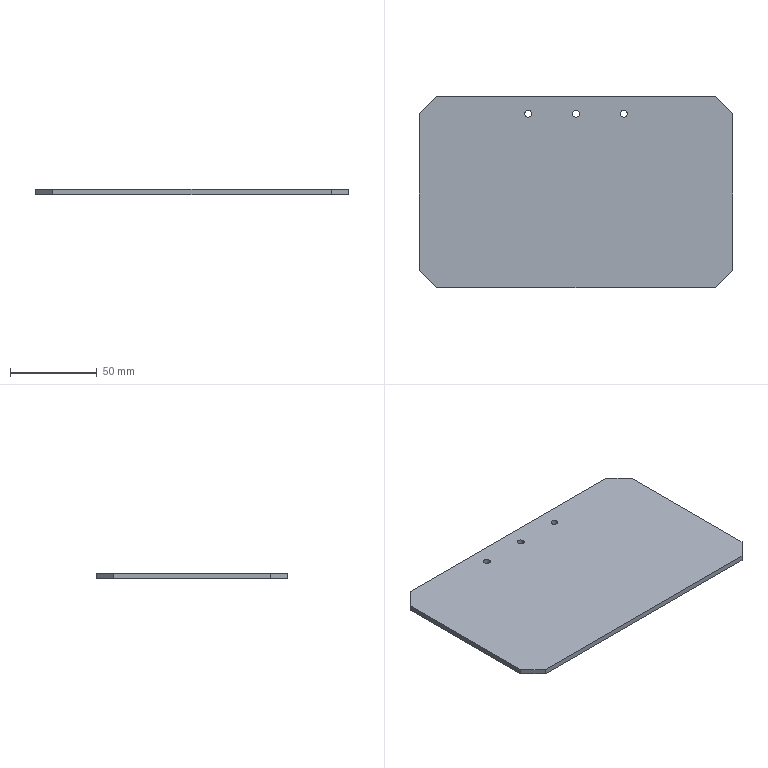Part | SolidWorks | features Extrusion 1 | 1 solid | 16 faces | box 180 x 110 x 3 mm | volume 58687 mm3 | plane 10 | cylinder 6 | commonest cylinder face diameters 4 x6
STEP:
#1=CARTESIAN_POINT('',(60.5,-10.,3.));
#2=VERTEX_POINT('',#1);
#3=CARTESIAN_POINT('',(64.5,-10.,3.));
#4=VERTEX_POINT('',#3);
#5=CARTESIAN_POINT('',(62.5,-10.,3.));
#6=DIRECTION('',(0.,0.,1.));
#7=DIRECTION('',(1.,0.,0.));
#8=AXIS2_PLACEMENT_3D('',#5,#6,#7);
#9=CIRCLE('',#8,2.);
#10=EDGE_CURVE('',#2,#4,#9,.T.);
#11=ORIENTED_EDGE('',*,*,#10,.T.);
#12=CARTESIAN_POINT('',(64.5,-10.,0.));
#13=VERTEX_POINT('',#12);
#14=CARTESIAN_POINT('',(64.5,-10.,3.));
#15=DIRECTION('',(0.,0.,-1.));
#16=VECTOR('',#15,1000.);
#17=LINE('',#14,#16);
#18=EDGE_CURVE('',#4,#13,#17,.T.);
#19=ORIENTED_EDGE('',*,*,#18,.T.);
#20=CARTESIAN_POINT('',(60.5,-10.,0.));
#21=VERTEX_POINT('',#20);
#22=CARTESIAN_POINT('',(62.5,-10.,0.));
#23=DIRECTION('',(0.,0.,1.));
#24=DIRECTION('',(1.,0.,0.));
#25=AXIS2_PLACEMENT_3D('',#22,#23,#24);
#26=CIRCLE('',#25,2.);
#27=EDGE_CURVE('',#21,#13,#26,.T.);
#28=ORIENTED_EDGE('',*,*,#27,.F.);
#29=CARTESIAN_POINT('',(60.5,-10.,3.));
#30=DIRECTION('',(0.,0.,-1.));
#31=VECTOR('',#30,1000.);
#32=LINE('',#29,#31);
#33=EDGE_CURVE('',#2,#21,#32,.T.);
#34=ORIENTED_EDGE('',*,*,#33,.F.);
#35=EDGE_LOOP('',(#11,#19,#28,#34));
#36=FACE_OUTER_BOUND('',#35,.T.);
#37=CARTESIAN_POINT('',(62.5,-10.,3.));
#38=DIRECTION('',(0.,0.,-1.));
#39=DIRECTION('',(-1.,0.,0.));
#40=AXIS2_PLACEMENT_3D('',#37,#38,#39);
#41=CYLINDRICAL_SURFACE('',#40,2.);
#42=ADVANCED_FACE('',(#36),#41,.F.);
#43=CARTESIAN_POINT('',(115.5,-10.,3.));
#44=VERTEX_POINT('',#43);
#45=CARTESIAN_POINT('',(119.5,-10.,3.));
#46=VERTEX_POINT('',#45);
#47=CARTESIAN_POINT('',(117.5,-10.,3.));
#48=DIRECTION('',(0.,0.,1.));
#49=DIRECTION('',(1.,0.,0.));
#50=AXIS2_PLACEMENT_3D('',#47,#48,#49);
#51=CIRCLE('',#50,2.);
#52=EDGE_CURVE('',#44,#46,#51,.T.);
#53=ORIENTED_EDGE('',*,*,#52,.T.);
#54=CARTESIAN_POINT('',(119.5,-10.,0.));
#55=VERTEX_POINT('',#54);
#56=CARTESIAN_POINT('',(119.5,-10.,3.));
#57=DIRECTION('',(0.,0.,-1.));
#58=VECTOR('',#57,1000.);
#59=LINE('',#56,#58);
#60=EDGE_CURVE('',#46,#55,#59,.T.);
#61=ORIENTED_EDGE('',*,*,#60,.T.);
#62=CARTESIAN_POINT('',(115.5,-10.,0.));
#63=VERTEX_POINT('',#62);
#64=CARTESIAN_POINT('',(117.5,-10.,0.));
#65=DIRECTION('',(0.,0.,1.));
#66=DIRECTION('',(1.,0.,0.));
#67=AXIS2_PLACEMENT_3D('',#64,#65,#66);
#68=CIRCLE('',#67,2.);
#69=EDGE_CURVE('',#63,#55,#68,.T.);
#70=ORIENTED_EDGE('',*,*,#69,.F.);
#71=CARTESIAN_POINT('',(115.5,-10.,3.));
#72=DIRECTION('',(0.,0.,-1.));
#73=VECTOR('',#72,1000.);
#74=LINE('',#71,#73);
#75=EDGE_CURVE('',#44,#63,#74,.T.);
#76=ORIENTED_EDGE('',*,*,#75,.F.);
#77=EDGE_LOOP('',(#53,#61,#70,#76));
#78=FACE_OUTER_BOUND('',#77,.T.);
#79=CARTESIAN_POINT('',(117.5,-10.,3.));
#80=DIRECTION('',(0.,0.,-1.));
#81=DIRECTION('',(-1.,0.,0.));
#82=AXIS2_PLACEMENT_3D('',#79,#80,#81);
#83=CYLINDRICAL_SURFACE('',#82,2.);
#84=ADVANCED_FACE('',(#78),#83,.F.);
#85=CARTESIAN_POINT('',(88.,-10.,3.));
#86=VERTEX_POINT('',#85);
#87=CARTESIAN_POINT('',(92.,-10.,3.));
#88=VERTEX_POINT('',#87);
#89=CARTESIAN_POINT('',(90.,-10.,3.));
#90=DIRECTION('',(0.,0.,1.));
#91=DIRECTION('',(1.,0.,0.));
#92=AXIS2_PLACEMENT_3D('',#89,#90,#91);
#93=CIRCLE('',#92,2.);
#94=EDGE_CURVE('',#86,#88,#93,.T.);
#95=ORIENTED_EDGE('',*,*,#94,.T.);
#96=CARTESIAN_POINT('',(92.,-10.,0.));
#97=VERTEX_POINT('',#96);
#98=CARTESIAN_POINT('',(92.,-10.,3.));
#99=DIRECTION('',(0.,0.,-1.));
#100=VECTOR('',#99,1000.);
#101=LINE('',#98,#100);
#102=EDGE_CURVE('',#88,#97,#101,.T.);
#103=ORIENTED_EDGE('',*,*,#102,.T.);
#104=CARTESIAN_POINT('',(88.,-10.,0.));
#105=VERTEX_POINT('',#104);
#106=CARTESIAN_POINT('',(90.,-10.,0.));
#107=DIRECTION('',(0.,0.,1.));
#108=DIRECTION('',(1.,0.,0.));
#109=AXIS2_PLACEMENT_3D('',#106,#107,#108);
#110=CIRCLE('',#109,2.);
#111=EDGE_CURVE('',#105,#97,#110,.T.);
#112=ORIENTED_EDGE('',*,*,#111,.F.);
#113=CARTESIAN_POINT('',(88.,-10.,3.));
#114=DIRECTION('',(0.,0.,-1.));
#115=VECTOR('',#114,1000.);
#116=LINE('',#113,#115);
#117=EDGE_CURVE('',#86,#105,#116,.T.);
#118=ORIENTED_EDGE('',*,*,#117,.F.);
#119=EDGE_LOOP('',(#95,#103,#112,#118));
#120=FACE_OUTER_BOUND('',#119,.T.);
#121=CARTESIAN_POINT('',(90.,-10.,3.));
#122=DIRECTION('',(0.,0.,-1.));
#123=DIRECTION('',(-1.,0.,0.));
#124=AXIS2_PLACEMENT_3D('',#121,#122,#123);
#125=CYLINDRICAL_SURFACE('',#124,2.);
#126=ADVANCED_FACE('',(#120),#125,.F.);
#127=ORIENTED_EDGE('',*,*,#52,.F.);
#128=CARTESIAN_POINT('',(117.5,-10.,3.));
#129=DIRECTION('',(0.,0.,1.));
#130=DIRECTION('',(1.,0.,0.));
#131=AXIS2_PLACEMENT_3D('',#128,#129,#130);
#132=CIRCLE('',#131,2.);
#133=EDGE_CURVE('',#46,#44,#132,.T.);
#134=ORIENTED_EDGE('',*,*,#133,.F.);
#135=EDGE_LOOP('',(#127,#134));
#136=FACE_BOUND('',#135,.T.);
#137=CARTESIAN_POINT('',(10.,0.,3.));
#138=VERTEX_POINT('',#137);
#139=CARTESIAN_POINT('',(0.,-10.,3.));
#140=VERTEX_POINT('',#139);
#141=CARTESIAN_POINT('',(10.,0.,3.));
#142=DIRECTION('',(-0.7071,-0.7071,0.));
#143=VECTOR('',#142,1000.);
#144=LINE('',#141,#143);
#145=EDGE_CURVE('',#138,#140,#144,.T.);
#146=ORIENTED_EDGE('',*,*,#145,.T.);
#147=CARTESIAN_POINT('',(0.,-100.,3.));
#148=VERTEX_POINT('',#147);
#149=CARTESIAN_POINT('',(0.,-10.,3.));
#150=DIRECTION('',(0.,-1.,0.));
#151=VECTOR('',#150,1000.);
#152=LINE('',#149,#151);
#153=EDGE_CURVE('',#140,#148,#152,.T.);
#154=ORIENTED_EDGE('',*,*,#153,.T.);
#155=CARTESIAN_POINT('',(10.,-110.,3.));
#156=VERTEX_POINT('',#155);
#157=CARTESIAN_POINT('',(0.,-100.,3.));
#158=DIRECTION('',(0.7071,-0.7071,0.));
#159=VECTOR('',#158,1000.);
#160=LINE('',#157,#159);
#161=EDGE_CURVE('',#148,#156,#160,.T.);
#162=ORIENTED_EDGE('',*,*,#161,.T.);
#163=CARTESIAN_POINT('',(170.,-110.,3.));
#164=VERTEX_POINT('',#163);
#165=CARTESIAN_POINT('',(10.,-110.,3.));
#166=DIRECTION('',(1.,0.,0.));
#167=VECTOR('',#166,1000.);
#168=LINE('',#165,#167);
#169=EDGE_CURVE('',#156,#164,#168,.T.);
#170=ORIENTED_EDGE('',*,*,#169,.T.);
#171=CARTESIAN_POINT('',(180.,-100.,3.));
#172=VERTEX_POINT('',#171);
#173=CARTESIAN_POINT('',(180.,-100.,3.));
#174=DIRECTION('',(0.7071,0.7071,0.));
#175=VECTOR('',#174,1000.);
#176=LINE('',#173,#175);
#177=EDGE_CURVE('',#164,#172,#176,.T.);
#178=ORIENTED_EDGE('',*,*,#177,.T.);
#179=CARTESIAN_POINT('',(180.,-10.,3.));
#180=VERTEX_POINT('',#179);
#181=CARTESIAN_POINT('',(180.,-10.,3.));
#182=DIRECTION('',(0.,1.,0.));
#183=VECTOR('',#182,1000.);
#184=LINE('',#181,#183);
#185=EDGE_CURVE('',#172,#180,#184,.T.);
#186=ORIENTED_EDGE('',*,*,#185,.T.);
#187=CARTESIAN_POINT('',(170.,0.,3.));
#188=VERTEX_POINT('',#187);
#189=CARTESIAN_POINT('',(170.,0.,3.));
#190=DIRECTION('',(-0.7071,0.7071,0.));
#191=VECTOR('',#190,1000.);
#192=LINE('',#189,#191);
#193=EDGE_CURVE('',#180,#188,#192,.T.);
#194=ORIENTED_EDGE('',*,*,#193,.T.);
#195=CARTESIAN_POINT('',(10.,0.,3.));
#196=DIRECTION('',(-1.,0.,0.));
#197=VECTOR('',#196,1000.);
#198=LINE('',#195,#197);
#199=EDGE_CURVE('',#188,#138,#198,.T.);
#200=ORIENTED_EDGE('',*,*,#199,.T.);
#201=EDGE_LOOP('',(#146,#154,#162,#170,#178,#186,#194,#200));
#202=FACE_OUTER_BOUND('',#201,.T.);
#203=ORIENTED_EDGE('',*,*,#94,.F.);
#204=CARTESIAN_POINT('',(90.,-10.,3.));
#205=DIRECTION('',(0.,0.,1.));
#206=DIRECTION('',(1.,0.,0.));
#207=AXIS2_PLACEMENT_3D('',#204,#205,#206);
#208=CIRCLE('',#207,2.);
#209=EDGE_CURVE('',#88,#86,#208,.T.);
#210=ORIENTED_EDGE('',*,*,#209,.F.);
#211=EDGE_LOOP('',(#203,#210));
#212=FACE_BOUND('',#211,.T.);
#213=ORIENTED_EDGE('',*,*,#10,.F.);
#214=CARTESIAN_POINT('',(62.5,-10.,3.));
#215=DIRECTION('',(0.,0.,1.));
#216=DIRECTION('',(1.,0.,0.));
#217=AXIS2_PLACEMENT_3D('',#214,#215,#216);
#218=CIRCLE('',#217,2.);
#219=EDGE_CURVE('',#4,#2,#218,.T.);
#220=ORIENTED_EDGE('',*,*,#219,.F.);
#221=EDGE_LOOP('',(#213,#220));
#222=FACE_BOUND('',#221,.T.);
#223=CARTESIAN_POINT('',(0.,0.,3.));
#224=DIRECTION('',(0.,0.,1.));
#225=DIRECTION('',(1.,0.,0.));
#226=AXIS2_PLACEMENT_3D('',#223,#224,#225);
#227=PLANE('',#226);
#228=ADVANCED_FACE('',(#136,#202,#212,#222),#227,.T.);
#229=CARTESIAN_POINT('',(10.,0.,0.));
#230=VERTEX_POINT('',#229);
#231=CARTESIAN_POINT('',(0.,-10.,0.));
#232=VERTEX_POINT('',#231);
#233=CARTESIAN_POINT('',(10.,0.,0.));
#234=DIRECTION('',(-0.7071,-0.7071,0.));
#235=VECTOR('',#234,1000.);
#236=LINE('',#233,#235);
#237=EDGE_CURVE('',#230,#232,#236,.T.);
#238=ORIENTED_EDGE('',*,*,#237,.F.);
#239=CARTESIAN_POINT('',(170.,0.,0.));
#240=VERTEX_POINT('',#239);
#241=CARTESIAN_POINT('',(10.,0.,0.));
#242=DIRECTION('',(-1.,0.,0.));
#243=VECTOR('',#242,1000.);
#244=LINE('',#241,#243);
#245=EDGE_CURVE('',#240,#230,#244,.T.);
#246=ORIENTED_EDGE('',*,*,#245,.F.);
#247=CARTESIAN_POINT('',(180.,-10.,0.));
#248=VERTEX_POINT('',#247);
#249=CARTESIAN_POINT('',(170.,0.,0.));
#250=DIRECTION('',(-0.7071,0.7071,0.));
#251=VECTOR('',#250,1000.);
#252=LINE('',#249,#251);
#253=EDGE_CURVE('',#248,#240,#252,.T.);
#254=ORIENTED_EDGE('',*,*,#253,.F.);
#255=CARTESIAN_POINT('',(180.,-100.,0.));
#256=VERTEX_POINT('',#255);
#257=CARTESIAN_POINT('',(180.,-10.,0.));
#258=DIRECTION('',(0.,1.,0.));
#259=VECTOR('',#258,1000.);
#260=LINE('',#257,#259);
#261=EDGE_CURVE('',#256,#248,#260,.T.);
#262=ORIENTED_EDGE('',*,*,#261,.F.);
#263=CARTESIAN_POINT('',(170.,-110.,0.));
#264=VERTEX_POINT('',#263);
#265=CARTESIAN_POINT('',(180.,-100.,0.));
#266=DIRECTION('',(0.7071,0.7071,0.));
#267=VECTOR('',#266,1000.);
#268=LINE('',#265,#267);
#269=EDGE_CURVE('',#264,#256,#268,.T.);
#270=ORIENTED_EDGE('',*,*,#269,.F.);
#271=CARTESIAN_POINT('',(10.,-110.,0.));
#272=VERTEX_POINT('',#271);
#273=CARTESIAN_POINT('',(10.,-110.,0.));
#274=DIRECTION('',(1.,0.,0.));
#275=VECTOR('',#274,1000.);
#276=LINE('',#273,#275);
#277=EDGE_CURVE('',#272,#264,#276,.T.);
#278=ORIENTED_EDGE('',*,*,#277,.F.);
#279=CARTESIAN_POINT('',(0.,-100.,0.));
#280=VERTEX_POINT('',#279);
#281=CARTESIAN_POINT('',(0.,-100.,0.));
#282=DIRECTION('',(0.7071,-0.7071,0.));
#283=VECTOR('',#282,1000.);
#284=LINE('',#281,#283);
#285=EDGE_CURVE('',#280,#272,#284,.T.);
#286=ORIENTED_EDGE('',*,*,#285,.F.);
#287=CARTESIAN_POINT('',(0.,-10.,0.));
#288=DIRECTION('',(0.,-1.,0.));
#289=VECTOR('',#288,1000.);
#290=LINE('',#287,#289);
#291=EDGE_CURVE('',#232,#280,#290,.T.);
#292=ORIENTED_EDGE('',*,*,#291,.F.);
#293=EDGE_LOOP('',(#238,#246,#254,#262,#270,#278,#286,#292));
#294=FACE_OUTER_BOUND('',#293,.T.);
#295=ORIENTED_EDGE('',*,*,#111,.T.);
#296=CARTESIAN_POINT('',(90.,-10.,0.));
#297=DIRECTION('',(0.,0.,1.));
#298=DIRECTION('',(1.,0.,0.));
#299=AXIS2_PLACEMENT_3D('',#296,#297,#298);
#300=CIRCLE('',#299,2.);
#301=EDGE_CURVE('',#97,#105,#300,.T.);
#302=ORIENTED_EDGE('',*,*,#301,.T.);
#303=EDGE_LOOP('',(#295,#302));
#304=FACE_BOUND('',#303,.T.);
#305=ORIENTED_EDGE('',*,*,#69,.T.);
#306=CARTESIAN_POINT('',(117.5,-10.,0.));
#307=DIRECTION('',(0.,0.,1.));
#308=DIRECTION('',(1.,0.,0.));
#309=AXIS2_PLACEMENT_3D('',#306,#307,#308);
#310=CIRCLE('',#309,2.);
#311=EDGE_CURVE('',#55,#63,#310,.T.);
#312=ORIENTED_EDGE('',*,*,#311,.T.);
#313=EDGE_LOOP('',(#305,#312));
#314=FACE_BOUND('',#313,.T.);
#315=ORIENTED_EDGE('',*,*,#27,.T.);
#316=CARTESIAN_POINT('',(62.5,-10.,0.));
#317=DIRECTION('',(0.,0.,1.));
#318=DIRECTION('',(1.,0.,0.));
#319=AXIS2_PLACEMENT_3D('',#316,#317,#318);
#320=CIRCLE('',#319,2.);
#321=EDGE_CURVE('',#13,#21,#320,.T.);
#322=ORIENTED_EDGE('',*,*,#321,.T.);
#323=EDGE_LOOP('',(#315,#322));
#324=FACE_BOUND('',#323,.T.);
#325=CARTESIAN_POINT('',(0.,0.,0.));
#326=DIRECTION('',(0.,0.,1.));
#327=DIRECTION('',(1.,0.,0.));
#328=AXIS2_PLACEMENT_3D('',#325,#326,#327);
#329=PLANE('',#328);
#330=ADVANCED_FACE('',(#294,#304,#314,#324),#329,.F.);
#331=ORIENTED_EDGE('',*,*,#237,.T.);
#332=CARTESIAN_POINT('',(0.,-10.,3.));
#333=DIRECTION('',(0.,0.,-1.));
#334=VECTOR('',#333,1000.);
#335=LINE('',#332,#334);
#336=EDGE_CURVE('',#140,#232,#335,.T.);
#337=ORIENTED_EDGE('',*,*,#336,.F.);
#338=ORIENTED_EDGE('',*,*,#145,.F.);
#339=CARTESIAN_POINT('',(10.,0.,3.));
#340=DIRECTION('',(0.,0.,-1.));
#341=VECTOR('',#340,1000.);
#342=LINE('',#339,#341);
#343=EDGE_CURVE('',#138,#230,#342,.T.);
#344=ORIENTED_EDGE('',*,*,#343,.T.);
#345=EDGE_LOOP('',(#331,#337,#338,#344));
#346=FACE_OUTER_BOUND('',#345,.T.);
#347=CARTESIAN_POINT('',(10.,0.,3.));
#348=DIRECTION('',(0.7071,-0.7071,0.));
#349=DIRECTION('',(0.7071,0.7071,0.));
#350=AXIS2_PLACEMENT_3D('',#347,#348,#349);
#351=PLANE('',#350);
#352=ADVANCED_FACE('',(#346),#351,.F.);
#353=ORIENTED_EDGE('',*,*,#291,.T.);
#354=CARTESIAN_POINT('',(0.,-100.,3.));
#355=DIRECTION('',(0.,0.,-1.));
#356=VECTOR('',#355,1000.);
#357=LINE('',#354,#356);
#358=EDGE_CURVE('',#148,#280,#357,.T.);
#359=ORIENTED_EDGE('',*,*,#358,.F.);
#360=ORIENTED_EDGE('',*,*,#153,.F.);
#361=ORIENTED_EDGE('',*,*,#336,.T.);
#362=EDGE_LOOP('',(#353,#359,#360,#361));
#363=FACE_OUTER_BOUND('',#362,.T.);
#364=CARTESIAN_POINT('',(0.,-10.,3.));
#365=DIRECTION('',(1.,0.,0.));
#366=DIRECTION('',(0.,1.,0.));
#367=AXIS2_PLACEMENT_3D('',#364,#365,#366);
#368=PLANE('',#367);
#369=ADVANCED_FACE('',(#363),#368,.F.);
#370=ORIENTED_EDGE('',*,*,#285,.T.);
#371=CARTESIAN_POINT('',(10.,-110.,3.));
#372=DIRECTION('',(0.,0.,-1.));
#373=VECTOR('',#372,1000.);
#374=LINE('',#371,#373);
#375=EDGE_CURVE('',#156,#272,#374,.T.);
#376=ORIENTED_EDGE('',*,*,#375,.F.);
#377=ORIENTED_EDGE('',*,*,#161,.F.);
#378=ORIENTED_EDGE('',*,*,#358,.T.);
#379=EDGE_LOOP('',(#370,#376,#377,#378));
#380=FACE_OUTER_BOUND('',#379,.T.);
#381=CARTESIAN_POINT('',(0.,-100.,3.));
#382=DIRECTION('',(0.7071,0.7071,0.));
#383=DIRECTION('',(-0.7071,0.7071,0.));
#384=AXIS2_PLACEMENT_3D('',#381,#382,#383);
#385=PLANE('',#384);
#386=ADVANCED_FACE('',(#380),#385,.F.);
#387=ORIENTED_EDGE('',*,*,#277,.T.);
#388=CARTESIAN_POINT('',(170.,-110.,3.));
#389=DIRECTION('',(0.,0.,-1.));
#390=VECTOR('',#389,1000.);
#391=LINE('',#388,#390);
#392=EDGE_CURVE('',#164,#264,#391,.T.);
#393=ORIENTED_EDGE('',*,*,#392,.F.);
#394=ORIENTED_EDGE('',*,*,#169,.F.);
#395=ORIENTED_EDGE('',*,*,#375,.T.);
#396=EDGE_LOOP('',(#387,#393,#394,#395));
#397=FACE_OUTER_BOUND('',#396,.T.);
#398=CARTESIAN_POINT('',(10.,-110.,3.));
#399=DIRECTION('',(0.,1.,0.));
#400=DIRECTION('',(0.,0.,1.));
#401=AXIS2_PLACEMENT_3D('',#398,#399,#400);
#402=PLANE('',#401);
#403=ADVANCED_FACE('',(#397),#402,.F.);
#404=ORIENTED_EDGE('',*,*,#269,.T.);
#405=CARTESIAN_POINT('',(180.,-100.,3.));
#406=DIRECTION('',(0.,0.,-1.));
#407=VECTOR('',#406,1000.);
#408=LINE('',#405,#407);
#409=EDGE_CURVE('',#172,#256,#408,.T.);
#410=ORIENTED_EDGE('',*,*,#409,.F.);
#411=ORIENTED_EDGE('',*,*,#177,.F.);
#412=ORIENTED_EDGE('',*,*,#392,.T.);
#413=EDGE_LOOP('',(#404,#410,#411,#412));
#414=FACE_OUTER_BOUND('',#413,.T.);
#415=CARTESIAN_POINT('',(180.,-100.,3.));
#416=DIRECTION('',(-0.7071,0.7071,0.));
#417=DIRECTION('',(-0.7071,-0.7071,0.));
#418=AXIS2_PLACEMENT_3D('',#415,#416,#417);
#419=PLANE('',#418);
#420=ADVANCED_FACE('',(#414),#419,.F.);
#421=ORIENTED_EDGE('',*,*,#261,.T.);
#422=CARTESIAN_POINT('',(180.,-10.,3.));
#423=DIRECTION('',(0.,0.,-1.));
#424=VECTOR('',#423,1000.);
#425=LINE('',#422,#424);
#426=EDGE_CURVE('',#180,#248,#425,.T.);
#427=ORIENTED_EDGE('',*,*,#426,.F.);
#428=ORIENTED_EDGE('',*,*,#185,.F.);
#429=ORIENTED_EDGE('',*,*,#409,.T.);
#430=EDGE_LOOP('',(#421,#427,#428,#429));
#431=FACE_OUTER_BOUND('',#430,.T.);
#432=CARTESIAN_POINT('',(180.,-10.,3.));
#433=DIRECTION('',(-1.,0.,0.));
#434=DIRECTION('',(0.,0.,1.));
#435=AXIS2_PLACEMENT_3D('',#432,#433,#434);
#436=PLANE('',#435);
#437=ADVANCED_FACE('',(#431),#436,.F.);
#438=ORIENTED_EDGE('',*,*,#253,.T.);
#439=CARTESIAN_POINT('',(170.,0.,3.));
#440=DIRECTION('',(0.,0.,-1.));
#441=VECTOR('',#440,1000.);
#442=LINE('',#439,#441);
#443=EDGE_CURVE('',#188,#240,#442,.T.);
#444=ORIENTED_EDGE('',*,*,#443,.F.);
#445=ORIENTED_EDGE('',*,*,#193,.F.);
#446=ORIENTED_EDGE('',*,*,#426,.T.);
#447=EDGE_LOOP('',(#438,#444,#445,#446));
#448=FACE_OUTER_BOUND('',#447,.T.);
#449=CARTESIAN_POINT('',(170.,0.,3.));
#450=DIRECTION('',(-0.7071,-0.7071,0.));
#451=DIRECTION('',(0.7071,-0.7071,0.));
#452=AXIS2_PLACEMENT_3D('',#449,#450,#451);
#453=PLANE('',#452);
#454=ADVANCED_FACE('',(#448),#453,.F.);
#455=ORIENTED_EDGE('',*,*,#245,.T.);
#456=ORIENTED_EDGE('',*,*,#343,.F.);
#457=ORIENTED_EDGE('',*,*,#199,.F.);
#458=ORIENTED_EDGE('',*,*,#443,.T.);
#459=EDGE_LOOP('',(#455,#456,#457,#458));
#460=FACE_OUTER_BOUND('',#459,.T.);
#461=CARTESIAN_POINT('',(10.,0.,3.));
#462=DIRECTION('',(0.,-1.,0.));
#463=DIRECTION('',(0.,0.,-1.));
#464=AXIS2_PLACEMENT_3D('',#461,#462,#463);
#465=PLANE('',#464);
#466=ADVANCED_FACE('',(#460),#465,.F.);
#467=ORIENTED_EDGE('',*,*,#102,.F.);
#468=ORIENTED_EDGE('',*,*,#209,.T.);
#469=ORIENTED_EDGE('',*,*,#117,.T.);
#470=ORIENTED_EDGE('',*,*,#301,.F.);
#471=EDGE_LOOP('',(#467,#468,#469,#470));
#472=FACE_OUTER_BOUND('',#471,.T.);
#473=CARTESIAN_POINT('',(90.,-10.,3.));
#474=DIRECTION('',(0.,0.,-1.));
#475=DIRECTION('',(-1.,0.,0.));
#476=AXIS2_PLACEMENT_3D('',#473,#474,#475);
#477=CYLINDRICAL_SURFACE('',#476,2.);
#478=ADVANCED_FACE('',(#472),#477,.F.);
#479=ORIENTED_EDGE('',*,*,#60,.F.);
#480=ORIENTED_EDGE('',*,*,#133,.T.);
#481=ORIENTED_EDGE('',*,*,#75,.T.);
#482=ORIENTED_EDGE('',*,*,#311,.F.);
#483=EDGE_LOOP('',(#479,#480,#481,#482));
#484=FACE_OUTER_BOUND('',#483,.T.);
#485=CARTESIAN_POINT('',(117.5,-10.,3.));
#486=DIRECTION('',(0.,0.,-1.));
#487=DIRECTION('',(-1.,0.,0.));
#488=AXIS2_PLACEMENT_3D('',#485,#486,#487);
#489=CYLINDRICAL_SURFACE('',#488,2.);
#490=ADVANCED_FACE('',(#484),#489,.F.);
#491=ORIENTED_EDGE('',*,*,#18,.F.);
#492=ORIENTED_EDGE('',*,*,#219,.T.);
#493=ORIENTED_EDGE('',*,*,#33,.T.);
#494=ORIENTED_EDGE('',*,*,#321,.F.);
#495=EDGE_LOOP('',(#491,#492,#493,#494));
#496=FACE_OUTER_BOUND('',#495,.T.);
#497=CARTESIAN_POINT('',(62.5,-10.,3.));
#498=DIRECTION('',(0.,0.,-1.));
#499=DIRECTION('',(-1.,0.,0.));
#500=AXIS2_PLACEMENT_3D('',#497,#498,#499);
#501=CYLINDRICAL_SURFACE('',#500,2.);
#502=ADVANCED_FACE('',(#496),#501,.F.);
#503=CLOSED_SHELL('',(#42,#84,#126,#228,#330,#352,#369,#386,#403,#420,#437,#454,#466,#478,#490,#502));
#504=MANIFOLD_SOLID_BREP('',#503);
#505=CARTESIAN_POINT('',(0.,0.,0.));
#506=DIRECTION('',(0.,0.,1.));
#507=DIRECTION('',(1.,0.,0.));
#508=AXIS2_PLACEMENT_3D('',#505,#506,#507);
#509=(LENGTH_UNIT()NAMED_UNIT(*)SI_UNIT(.MILLI.,.METRE.));
#510=UNCERTAINTY_MEASURE_WITH_UNIT(LENGTH_MEASURE(0.00001),#509,'','');
#511=(NAMED_UNIT(*)PLANE_ANGLE_UNIT()SI_UNIT($,.RADIAN.));
#512=(NAMED_UNIT(*)SI_UNIT($,.STERADIAN.)SOLID_ANGLE_UNIT());
#513=(GEOMETRIC_REPRESENTATION_CONTEXT(3)GLOBAL_UNCERTAINTY_ASSIGNED_CONTEXT((#510))GLOBAL_UNIT_ASSIGNED_CONTEXT((#509,#511,#512))REPRESENTATION_CONTEXT('',''));
#514=ADVANCED_BREP_SHAPE_REPRESENTATION('',(#504,#508),#513);